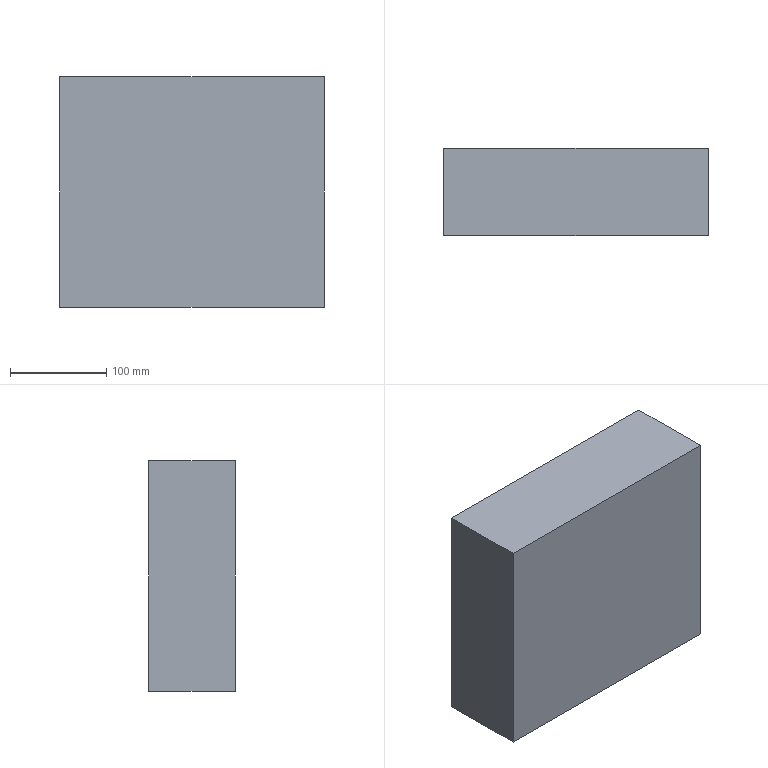Part | STEP file | UPS | 1 solid | 6 faces | box 275 x 90 x 240 mm | volume 5940000 mm3 | plane 6
STEP:
#1=CARTESIAN_POINT('',(0.,0.,0.));
#2=DIRECTION('',(0.,0.,1.));
#3=DIRECTION('',(1.,0.,0.));
#4=AXIS2_PLACEMENT_3D('',#1,#2,#3);
#5=CARTESIAN_POINT('',(-137.5,-45.,-120.));
#6=VERTEX_POINT('',#5);
#7=CARTESIAN_POINT('',(-137.5,-45.,120.));
#8=VERTEX_POINT('',#7);
#9=CARTESIAN_POINT('',(-137.5,-45.,-120.));
#10=DIRECTION('',(0.,0.,1.));
#11=VECTOR('',#10,1.);
#12=LINE('',#9,#11);
#13=CARTESIAN_POINT('',(-137.5,45.,-120.));
#14=DIRECTION('',(1.,0.,0.));
#15=DIRECTION('',(0.,0.,-1.));
#16=AXIS2_PLACEMENT_3D('',#13,#14,#15);
#17=PLANE('',#16);
#18=CARTESIAN_POINT('',(0.,-90.));
#19=DIRECTION('',(-1.,0.));
#20=VECTOR('',#19,1.);
#21=LINE('',#18,#20);
#22=(GEOMETRIC_REPRESENTATION_CONTEXT(2)PARAMETRIC_REPRESENTATION_CONTEXT()REPRESENTATION_CONTEXT('',''));
#23=DEFINITIONAL_REPRESENTATION('',(#21),#22);
#24=PCURVE('',#17,#23);
#25=CARTESIAN_POINT('',(0.,-45.,0.));
#26=DIRECTION('',(0.,1.,0.));
#27=DIRECTION('',(0.,0.,1.));
#28=AXIS2_PLACEMENT_3D('',#25,#26,#27);
#29=PLANE('',#28);
#30=CARTESIAN_POINT('',(-120.,-137.5));
#31=DIRECTION('',(1.,0.));
#32=VECTOR('',#31,1.);
#33=LINE('',#30,#32);
#34=(GEOMETRIC_REPRESENTATION_CONTEXT(2)PARAMETRIC_REPRESENTATION_CONTEXT()REPRESENTATION_CONTEXT('',''));
#35=DEFINITIONAL_REPRESENTATION('',(#33),#34);
#36=PCURVE('',#29,#35);
#37=SURFACE_CURVE('',#12,(#24,#36),.PCURVE_S1.);
#38=EDGE_CURVE('',#6,#8,#37,.T.);
#39=ORIENTED_EDGE('',*,*,#38,.T.);
#40=CARTESIAN_POINT('',(-137.5,45.,120.));
#41=VERTEX_POINT('',#40);
#42=CARTESIAN_POINT('',(-137.5,45.,120.));
#43=DIRECTION('',(0.,-1.,0.));
#44=VECTOR('',#43,1.);
#45=LINE('',#42,#44);
#46=CARTESIAN_POINT('',(-240.,0.));
#47=DIRECTION('',(0.,-1.));
#48=VECTOR('',#47,1.);
#49=LINE('',#46,#48);
#50=(GEOMETRIC_REPRESENTATION_CONTEXT(2)PARAMETRIC_REPRESENTATION_CONTEXT()REPRESENTATION_CONTEXT('',''));
#51=DEFINITIONAL_REPRESENTATION('',(#49),#50);
#52=PCURVE('',#17,#51);
#53=CARTESIAN_POINT('',(-137.5,45.,120.));
#54=DIRECTION('',(0.,0.,-1.));
#55=DIRECTION('',(-1.,0.,0.));
#56=AXIS2_PLACEMENT_3D('',#53,#54,#55);
#57=PLANE('',#56);
#58=CARTESIAN_POINT('',(0.,0.));
#59=DIRECTION('',(0.,-1.));
#60=VECTOR('',#59,1.);
#61=LINE('',#58,#60);
#62=(GEOMETRIC_REPRESENTATION_CONTEXT(2)PARAMETRIC_REPRESENTATION_CONTEXT()REPRESENTATION_CONTEXT('',''));
#63=DEFINITIONAL_REPRESENTATION('',(#61),#62);
#64=PCURVE('',#57,#63);
#65=SURFACE_CURVE('',#45,(#52,#64),.PCURVE_S1.);
#66=EDGE_CURVE('',#41,#8,#65,.T.);
#67=ORIENTED_EDGE('',*,*,#66,.F.);
#68=CARTESIAN_POINT('',(-137.5,45.,-120.));
#69=VERTEX_POINT('',#68);
#70=CARTESIAN_POINT('',(-137.5,45.,-120.));
#71=DIRECTION('',(0.,0.,1.));
#72=VECTOR('',#71,1.);
#73=LINE('',#70,#72);
#74=CARTESIAN_POINT('',(0.,0.));
#75=DIRECTION('',(-1.,0.));
#76=VECTOR('',#75,1.);
#77=LINE('',#74,#76);
#78=(GEOMETRIC_REPRESENTATION_CONTEXT(2)PARAMETRIC_REPRESENTATION_CONTEXT()REPRESENTATION_CONTEXT('',''));
#79=DEFINITIONAL_REPRESENTATION('',(#77),#78);
#80=PCURVE('',#17,#79);
#81=CARTESIAN_POINT('',(0.,45.,0.));
#82=DIRECTION('',(0.,1.,0.));
#83=DIRECTION('',(0.,0.,1.));
#84=AXIS2_PLACEMENT_3D('',#81,#82,#83);
#85=PLANE('',#84);
#86=CARTESIAN_POINT('',(-120.,-137.5));
#87=DIRECTION('',(1.,0.));
#88=VECTOR('',#87,1.);
#89=LINE('',#86,#88);
#90=(GEOMETRIC_REPRESENTATION_CONTEXT(2)PARAMETRIC_REPRESENTATION_CONTEXT()REPRESENTATION_CONTEXT('',''));
#91=DEFINITIONAL_REPRESENTATION('',(#89),#90);
#92=PCURVE('',#85,#91);
#93=SURFACE_CURVE('',#73,(#80,#92),.PCURVE_S1.);
#94=EDGE_CURVE('',#69,#41,#93,.T.);
#95=ORIENTED_EDGE('',*,*,#94,.F.);
#96=CARTESIAN_POINT('',(-137.5,45.,-120.));
#97=DIRECTION('',(0.,-1.,0.));
#98=VECTOR('',#97,1.);
#99=LINE('',#96,#98);
#100=CARTESIAN_POINT('',(0.,0.));
#101=DIRECTION('',(0.,-1.));
#102=VECTOR('',#101,1.);
#103=LINE('',#100,#102);
#104=(GEOMETRIC_REPRESENTATION_CONTEXT(2)PARAMETRIC_REPRESENTATION_CONTEXT()REPRESENTATION_CONTEXT('',''));
#105=DEFINITIONAL_REPRESENTATION('',(#103),#104);
#106=PCURVE('',#17,#105);
#107=CARTESIAN_POINT('',(-137.5,45.,-120.));
#108=DIRECTION('',(0.,0.,1.));
#109=DIRECTION('',(1.,0.,0.));
#110=AXIS2_PLACEMENT_3D('',#107,#108,#109);
#111=PLANE('',#110);
#112=CARTESIAN_POINT('',(0.,0.));
#113=DIRECTION('',(0.,-1.));
#114=VECTOR('',#113,1.);
#115=LINE('',#112,#114);
#116=(GEOMETRIC_REPRESENTATION_CONTEXT(2)PARAMETRIC_REPRESENTATION_CONTEXT()REPRESENTATION_CONTEXT('',''));
#117=DEFINITIONAL_REPRESENTATION('',(#115),#116);
#118=PCURVE('',#111,#117);
#119=SURFACE_CURVE('',#99,(#106,#118),.PCURVE_S1.);
#120=EDGE_CURVE('',#69,#6,#119,.T.);
#121=ORIENTED_EDGE('',*,*,#120,.T.);
#122=EDGE_LOOP('',(#39,#67,#95,#121));
#123=FACE_BOUND('',#122,.T.);
#124=ADVANCED_FACE('',(#123),#17,.F.);
#125=CARTESIAN_POINT('',(137.5,-45.,120.));
#126=VERTEX_POINT('',#125);
#127=CARTESIAN_POINT('',(-137.5,-45.,120.));
#128=DIRECTION('',(1.,0.,0.));
#129=VECTOR('',#128,1.);
#130=LINE('',#127,#129);
#131=CARTESIAN_POINT('',(0.,-90.));
#132=DIRECTION('',(-1.,0.));
#133=VECTOR('',#132,1.);
#134=LINE('',#131,#133);
#135=(GEOMETRIC_REPRESENTATION_CONTEXT(2)PARAMETRIC_REPRESENTATION_CONTEXT()REPRESENTATION_CONTEXT('',''));
#136=DEFINITIONAL_REPRESENTATION('',(#134),#135);
#137=PCURVE('',#57,#136);
#138=CARTESIAN_POINT('',(120.,-137.5));
#139=DIRECTION('',(0.,1.));
#140=VECTOR('',#139,1.);
#141=LINE('',#138,#140);
#142=(GEOMETRIC_REPRESENTATION_CONTEXT(2)PARAMETRIC_REPRESENTATION_CONTEXT()REPRESENTATION_CONTEXT('',''));
#143=DEFINITIONAL_REPRESENTATION('',(#141),#142);
#144=PCURVE('',#29,#143);
#145=SURFACE_CURVE('',#130,(#137,#144),.PCURVE_S1.);
#146=EDGE_CURVE('',#8,#126,#145,.T.);
#147=ORIENTED_EDGE('',*,*,#146,.T.);
#148=CARTESIAN_POINT('',(137.5,45.,120.));
#149=VERTEX_POINT('',#148);
#150=CARTESIAN_POINT('',(137.5,45.,120.));
#151=DIRECTION('',(0.,-1.,0.));
#152=VECTOR('',#151,1.);
#153=LINE('',#150,#152);
#154=CARTESIAN_POINT('',(-275.,0.));
#155=DIRECTION('',(0.,-1.));
#156=VECTOR('',#155,1.);
#157=LINE('',#154,#156);
#158=(GEOMETRIC_REPRESENTATION_CONTEXT(2)PARAMETRIC_REPRESENTATION_CONTEXT()REPRESENTATION_CONTEXT('',''));
#159=DEFINITIONAL_REPRESENTATION('',(#157),#158);
#160=PCURVE('',#57,#159);
#161=CARTESIAN_POINT('',(137.5,45.,-120.));
#162=DIRECTION('',(-1.,0.,0.));
#163=DIRECTION('',(0.,0.,1.));
#164=AXIS2_PLACEMENT_3D('',#161,#162,#163);
#165=PLANE('',#164);
#166=CARTESIAN_POINT('',(240.,0.));
#167=DIRECTION('',(0.,-1.));
#168=VECTOR('',#167,1.);
#169=LINE('',#166,#168);
#170=(GEOMETRIC_REPRESENTATION_CONTEXT(2)PARAMETRIC_REPRESENTATION_CONTEXT()REPRESENTATION_CONTEXT('',''));
#171=DEFINITIONAL_REPRESENTATION('',(#169),#170);
#172=PCURVE('',#165,#171);
#173=SURFACE_CURVE('',#153,(#160,#172),.PCURVE_S1.);
#174=EDGE_CURVE('',#149,#126,#173,.T.);
#175=ORIENTED_EDGE('',*,*,#174,.F.);
#176=CARTESIAN_POINT('',(-137.5,45.,120.));
#177=DIRECTION('',(1.,0.,0.));
#178=VECTOR('',#177,1.);
#179=LINE('',#176,#178);
#180=CARTESIAN_POINT('',(0.,0.));
#181=DIRECTION('',(-1.,0.));
#182=VECTOR('',#181,1.);
#183=LINE('',#180,#182);
#184=(GEOMETRIC_REPRESENTATION_CONTEXT(2)PARAMETRIC_REPRESENTATION_CONTEXT()REPRESENTATION_CONTEXT('',''));
#185=DEFINITIONAL_REPRESENTATION('',(#183),#184);
#186=PCURVE('',#57,#185);
#187=CARTESIAN_POINT('',(120.,-137.5));
#188=DIRECTION('',(0.,1.));
#189=VECTOR('',#188,1.);
#190=LINE('',#187,#189);
#191=(GEOMETRIC_REPRESENTATION_CONTEXT(2)PARAMETRIC_REPRESENTATION_CONTEXT()REPRESENTATION_CONTEXT('',''));
#192=DEFINITIONAL_REPRESENTATION('',(#190),#191);
#193=PCURVE('',#85,#192);
#194=SURFACE_CURVE('',#179,(#186,#193),.PCURVE_S1.);
#195=EDGE_CURVE('',#41,#149,#194,.T.);
#196=ORIENTED_EDGE('',*,*,#195,.F.);
#197=ORIENTED_EDGE('',*,*,#66,.T.);
#198=EDGE_LOOP('',(#147,#175,#196,#197));
#199=FACE_BOUND('',#198,.T.);
#200=ADVANCED_FACE('',(#199),#57,.F.);
#201=CARTESIAN_POINT('',(137.5,-45.,-120.));
#202=VERTEX_POINT('',#201);
#203=CARTESIAN_POINT('',(137.5,-45.,-120.));
#204=DIRECTION('',(0.,0.,-1.));
#205=VECTOR('',#204,1.);
#206=LINE('',#203,#205);
#207=CARTESIAN_POINT('',(0.,-90.));
#208=DIRECTION('',(-1.,0.));
#209=VECTOR('',#208,1.);
#210=LINE('',#207,#209);
#211=(GEOMETRIC_REPRESENTATION_CONTEXT(2)PARAMETRIC_REPRESENTATION_CONTEXT()REPRESENTATION_CONTEXT('',''));
#212=DEFINITIONAL_REPRESENTATION('',(#210),#211);
#213=PCURVE('',#165,#212);
#214=CARTESIAN_POINT('',(-120.,137.5));
#215=DIRECTION('',(-1.,0.));
#216=VECTOR('',#215,1.);
#217=LINE('',#214,#216);
#218=(GEOMETRIC_REPRESENTATION_CONTEXT(2)PARAMETRIC_REPRESENTATION_CONTEXT()REPRESENTATION_CONTEXT('',''));
#219=DEFINITIONAL_REPRESENTATION('',(#217),#218);
#220=PCURVE('',#29,#219);
#221=SURFACE_CURVE('',#206,(#213,#220),.PCURVE_S1.);
#222=EDGE_CURVE('',#126,#202,#221,.T.);
#223=ORIENTED_EDGE('',*,*,#222,.T.);
#224=CARTESIAN_POINT('',(137.5,45.,-120.));
#225=VERTEX_POINT('',#224);
#226=CARTESIAN_POINT('',(137.5,45.,-120.));
#227=DIRECTION('',(0.,-1.,0.));
#228=VECTOR('',#227,1.);
#229=LINE('',#226,#228);
#230=CARTESIAN_POINT('',(0.,0.));
#231=DIRECTION('',(0.,-1.));
#232=VECTOR('',#231,1.);
#233=LINE('',#230,#232);
#234=(GEOMETRIC_REPRESENTATION_CONTEXT(2)PARAMETRIC_REPRESENTATION_CONTEXT()REPRESENTATION_CONTEXT('',''));
#235=DEFINITIONAL_REPRESENTATION('',(#233),#234);
#236=PCURVE('',#165,#235);
#237=CARTESIAN_POINT('',(275.,0.));
#238=DIRECTION('',(0.,-1.));
#239=VECTOR('',#238,1.);
#240=LINE('',#237,#239);
#241=(GEOMETRIC_REPRESENTATION_CONTEXT(2)PARAMETRIC_REPRESENTATION_CONTEXT()REPRESENTATION_CONTEXT('',''));
#242=DEFINITIONAL_REPRESENTATION('',(#240),#241);
#243=PCURVE('',#111,#242);
#244=SURFACE_CURVE('',#229,(#236,#243),.PCURVE_S1.);
#245=EDGE_CURVE('',#225,#202,#244,.T.);
#246=ORIENTED_EDGE('',*,*,#245,.F.);
#247=CARTESIAN_POINT('',(137.5,45.,-120.));
#248=DIRECTION('',(0.,0.,-1.));
#249=VECTOR('',#248,1.);
#250=LINE('',#247,#249);
#251=CARTESIAN_POINT('',(0.,0.));
#252=DIRECTION('',(-1.,0.));
#253=VECTOR('',#252,1.);
#254=LINE('',#251,#253);
#255=(GEOMETRIC_REPRESENTATION_CONTEXT(2)PARAMETRIC_REPRESENTATION_CONTEXT()REPRESENTATION_CONTEXT('',''));
#256=DEFINITIONAL_REPRESENTATION('',(#254),#255);
#257=PCURVE('',#165,#256);
#258=CARTESIAN_POINT('',(-120.,137.5));
#259=DIRECTION('',(-1.,0.));
#260=VECTOR('',#259,1.);
#261=LINE('',#258,#260);
#262=(GEOMETRIC_REPRESENTATION_CONTEXT(2)PARAMETRIC_REPRESENTATION_CONTEXT()REPRESENTATION_CONTEXT('',''));
#263=DEFINITIONAL_REPRESENTATION('',(#261),#262);
#264=PCURVE('',#85,#263);
#265=SURFACE_CURVE('',#250,(#257,#264),.PCURVE_S1.);
#266=EDGE_CURVE('',#149,#225,#265,.T.);
#267=ORIENTED_EDGE('',*,*,#266,.F.);
#268=ORIENTED_EDGE('',*,*,#174,.T.);
#269=EDGE_LOOP('',(#223,#246,#267,#268));
#270=FACE_BOUND('',#269,.T.);
#271=ADVANCED_FACE('',(#270),#165,.F.);
#272=CARTESIAN_POINT('',(-137.5,-45.,-120.));
#273=DIRECTION('',(-1.,0.,0.));
#274=VECTOR('',#273,1.);
#275=LINE('',#272,#274);
#276=CARTESIAN_POINT('',(0.,-90.));
#277=DIRECTION('',(-1.,0.));
#278=VECTOR('',#277,1.);
#279=LINE('',#276,#278);
#280=(GEOMETRIC_REPRESENTATION_CONTEXT(2)PARAMETRIC_REPRESENTATION_CONTEXT()REPRESENTATION_CONTEXT('',''));
#281=DEFINITIONAL_REPRESENTATION('',(#279),#280);
#282=PCURVE('',#111,#281);
#283=CARTESIAN_POINT('',(-120.,-137.5));
#284=DIRECTION('',(0.,-1.));
#285=VECTOR('',#284,1.);
#286=LINE('',#283,#285);
#287=(GEOMETRIC_REPRESENTATION_CONTEXT(2)PARAMETRIC_REPRESENTATION_CONTEXT()REPRESENTATION_CONTEXT('',''));
#288=DEFINITIONAL_REPRESENTATION('',(#286),#287);
#289=PCURVE('',#29,#288);
#290=SURFACE_CURVE('',#275,(#282,#289),.PCURVE_S1.);
#291=EDGE_CURVE('',#202,#6,#290,.T.);
#292=ORIENTED_EDGE('',*,*,#291,.T.);
#293=ORIENTED_EDGE('',*,*,#120,.F.);
#294=CARTESIAN_POINT('',(-137.5,45.,-120.));
#295=DIRECTION('',(-1.,0.,0.));
#296=VECTOR('',#295,1.);
#297=LINE('',#294,#296);
#298=CARTESIAN_POINT('',(0.,0.));
#299=DIRECTION('',(-1.,0.));
#300=VECTOR('',#299,1.);
#301=LINE('',#298,#300);
#302=(GEOMETRIC_REPRESENTATION_CONTEXT(2)PARAMETRIC_REPRESENTATION_CONTEXT()REPRESENTATION_CONTEXT('',''));
#303=DEFINITIONAL_REPRESENTATION('',(#301),#302);
#304=PCURVE('',#111,#303);
#305=CARTESIAN_POINT('',(-120.,-137.5));
#306=DIRECTION('',(0.,-1.));
#307=VECTOR('',#306,1.);
#308=LINE('',#305,#307);
#309=(GEOMETRIC_REPRESENTATION_CONTEXT(2)PARAMETRIC_REPRESENTATION_CONTEXT()REPRESENTATION_CONTEXT('',''));
#310=DEFINITIONAL_REPRESENTATION('',(#308),#309);
#311=PCURVE('',#85,#310);
#312=SURFACE_CURVE('',#297,(#304,#311),.PCURVE_S1.);
#313=EDGE_CURVE('',#225,#69,#312,.T.);
#314=ORIENTED_EDGE('',*,*,#313,.F.);
#315=ORIENTED_EDGE('',*,*,#245,.T.);
#316=EDGE_LOOP('',(#292,#293,#314,#315));
#317=FACE_BOUND('',#316,.T.);
#318=ADVANCED_FACE('',(#317),#111,.F.);
#319=ORIENTED_EDGE('',*,*,#94,.T.);
#320=ORIENTED_EDGE('',*,*,#195,.T.);
#321=ORIENTED_EDGE('',*,*,#266,.T.);
#322=ORIENTED_EDGE('',*,*,#313,.T.);
#323=EDGE_LOOP('',(#319,#320,#321,#322));
#324=FACE_BOUND('',#323,.T.);
#325=ADVANCED_FACE('',(#324),#85,.T.);
#326=ORIENTED_EDGE('',*,*,#38,.F.);
#327=ORIENTED_EDGE('',*,*,#291,.F.);
#328=ORIENTED_EDGE('',*,*,#222,.F.);
#329=ORIENTED_EDGE('',*,*,#146,.F.);
#330=EDGE_LOOP('',(#326,#327,#328,#329));
#331=FACE_BOUND('',#330,.T.);
#332=ADVANCED_FACE('',(#331),#29,.F.);
#333=CLOSED_SHELL('',(#124,#200,#271,#318,#325,#332));
#334=MANIFOLD_SOLID_BREP('',#333);
#335=(LENGTH_UNIT()NAMED_UNIT(*)SI_UNIT(.MILLI.,.METRE.));
#336=UNCERTAINTY_MEASURE_WITH_UNIT(LENGTH_MEASURE(0.0000001),#335,'','');
#337=(NAMED_UNIT(*)PLANE_ANGLE_UNIT()SI_UNIT($,.RADIAN.));
#338=(NAMED_UNIT(*)SI_UNIT($,.STERADIAN.)SOLID_ANGLE_UNIT());
#339=(GEOMETRIC_REPRESENTATION_CONTEXT(3)GLOBAL_UNCERTAINTY_ASSIGNED_CONTEXT((#336))GLOBAL_UNIT_ASSIGNED_CONTEXT((#335,#337,#338))REPRESENTATION_CONTEXT('',''));
#340=ADVANCED_BREP_SHAPE_REPRESENTATION('',(#4,#334),#339);